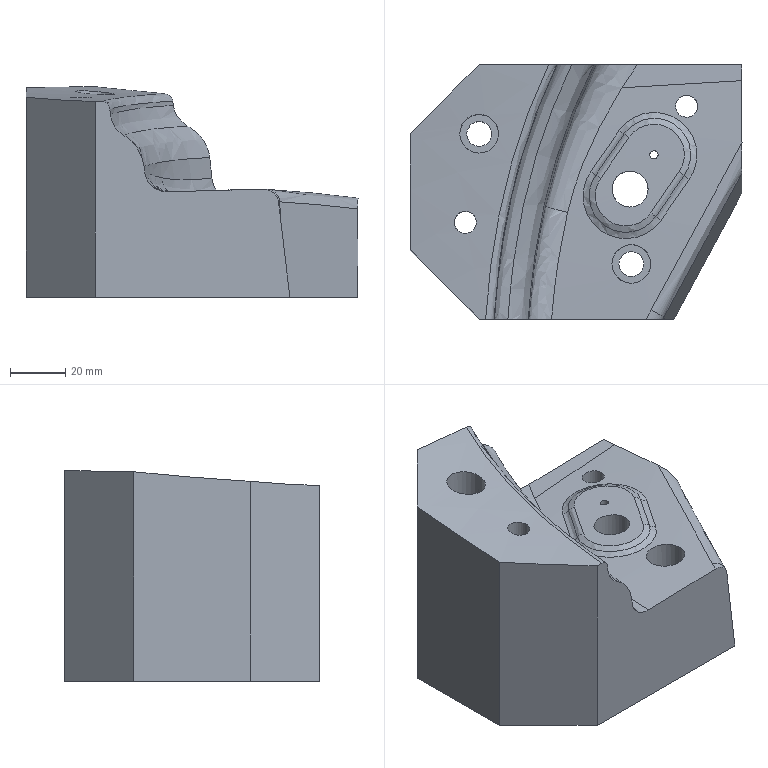Part | NX | features solid 2 | 1 solid | 40 faces | box 120.013 x 92 x 76.06 mm | volume 465452 mm3 | spline 21 | plane 10 | cylinder 9 | commonest cylinder face diameters 8 x2 9 x2 14 x2 3 x1 13 x1 322 x1